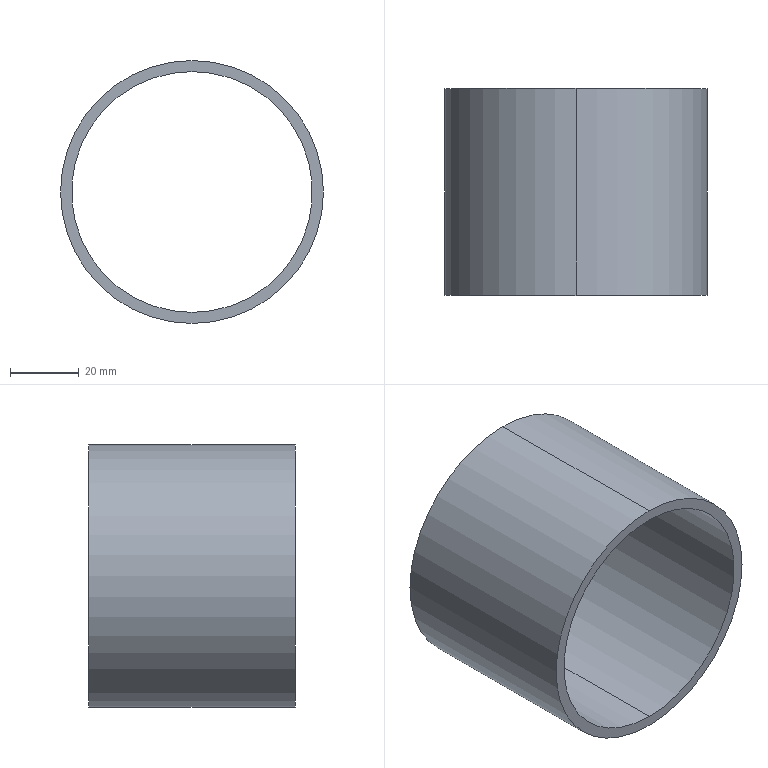Part | SolidWorks | features Extrusion 1 | 1 solid | 6 faces | box 76.3 x 60 x 76.3 mm | volume 44093 mm3 | cylinder 4 | plane 2 | commonest cylinder face diameters 69.9 x2 76.3 x2
STEP:
#1=CARTESIAN_POINT('',(0.,60.,-34.95));
#2=VERTEX_POINT('',#1);
#3=CARTESIAN_POINT('',(0.,60.,34.95));
#4=VERTEX_POINT('',#3);
#5=CARTESIAN_POINT('',(0.,60.,0.));
#6=DIRECTION('',(0.,1.,0.));
#7=DIRECTION('',(0.,0.,1.));
#8=AXIS2_PLACEMENT_3D('',#5,#6,#7);
#9=CIRCLE('',#8,34.95);
#10=EDGE_CURVE('',#2,#4,#9,.T.);
#11=ORIENTED_EDGE('',*,*,#10,.T.);
#12=CARTESIAN_POINT('',(0.,0.,34.95));
#13=VERTEX_POINT('',#12);
#14=CARTESIAN_POINT('',(0.,60.,34.95));
#15=DIRECTION('',(0.,-1.,0.));
#16=VECTOR('',#15,1000.);
#17=LINE('',#14,#16);
#18=EDGE_CURVE('',#4,#13,#17,.T.);
#19=ORIENTED_EDGE('',*,*,#18,.T.);
#20=CARTESIAN_POINT('',(0.,0.,-34.95));
#21=VERTEX_POINT('',#20);
#22=CARTESIAN_POINT('',(0.,0.,0.));
#23=DIRECTION('',(0.,1.,0.));
#24=DIRECTION('',(0.,0.,1.));
#25=AXIS2_PLACEMENT_3D('',#22,#23,#24);
#26=CIRCLE('',#25,34.95);
#27=EDGE_CURVE('',#21,#13,#26,.T.);
#28=ORIENTED_EDGE('',*,*,#27,.F.);
#29=CARTESIAN_POINT('',(0.,60.,-34.95));
#30=DIRECTION('',(0.,-1.,0.));
#31=VECTOR('',#30,1000.);
#32=LINE('',#29,#31);
#33=EDGE_CURVE('',#2,#21,#32,.T.);
#34=ORIENTED_EDGE('',*,*,#33,.F.);
#35=EDGE_LOOP('',(#11,#19,#28,#34));
#36=FACE_OUTER_BOUND('',#35,.T.);
#37=CARTESIAN_POINT('',(0.,60.,0.));
#38=DIRECTION('',(0.,-1.,0.));
#39=DIRECTION('',(0.,0.,-1.));
#40=AXIS2_PLACEMENT_3D('',#37,#38,#39);
#41=CYLINDRICAL_SURFACE('',#40,34.95);
#42=ADVANCED_FACE('',(#36),#41,.F.);
#43=CARTESIAN_POINT('',(0.,60.,38.15));
#44=VERTEX_POINT('',#43);
#45=CARTESIAN_POINT('',(0.,60.,-38.15));
#46=VERTEX_POINT('',#45);
#47=CARTESIAN_POINT('',(0.,60.,0.));
#48=DIRECTION('',(0.,1.,0.));
#49=DIRECTION('',(0.,0.,1.));
#50=AXIS2_PLACEMENT_3D('',#47,#48,#49);
#51=CIRCLE('',#50,38.15);
#52=EDGE_CURVE('',#44,#46,#51,.T.);
#53=ORIENTED_EDGE('',*,*,#52,.F.);
#54=CARTESIAN_POINT('',(0.,0.,38.15));
#55=VERTEX_POINT('',#54);
#56=CARTESIAN_POINT('',(0.,60.,38.15));
#57=DIRECTION('',(0.,-1.,0.));
#58=VECTOR('',#57,1000.);
#59=LINE('',#56,#58);
#60=EDGE_CURVE('',#44,#55,#59,.T.);
#61=ORIENTED_EDGE('',*,*,#60,.T.);
#62=CARTESIAN_POINT('',(0.,0.,-38.15));
#63=VERTEX_POINT('',#62);
#64=CARTESIAN_POINT('',(0.,0.,0.));
#65=DIRECTION('',(0.,1.,0.));
#66=DIRECTION('',(0.,0.,1.));
#67=AXIS2_PLACEMENT_3D('',#64,#65,#66);
#68=CIRCLE('',#67,38.15);
#69=EDGE_CURVE('',#55,#63,#68,.T.);
#70=ORIENTED_EDGE('',*,*,#69,.T.);
#71=CARTESIAN_POINT('',(0.,60.,-38.15));
#72=DIRECTION('',(0.,-1.,0.));
#73=VECTOR('',#72,1000.);
#74=LINE('',#71,#73);
#75=EDGE_CURVE('',#46,#63,#74,.T.);
#76=ORIENTED_EDGE('',*,*,#75,.F.);
#77=EDGE_LOOP('',(#53,#61,#70,#76));
#78=FACE_OUTER_BOUND('',#77,.T.);
#79=CARTESIAN_POINT('',(0.,60.,0.));
#80=DIRECTION('',(0.,-1.,0.));
#81=DIRECTION('',(0.,0.,-1.));
#82=AXIS2_PLACEMENT_3D('',#79,#80,#81);
#83=CYLINDRICAL_SURFACE('',#82,38.15);
#84=ADVANCED_FACE('',(#78),#83,.T.);
#85=CARTESIAN_POINT('',(0.,60.,0.));
#86=DIRECTION('',(0.,1.,0.));
#87=DIRECTION('',(0.,0.,1.));
#88=AXIS2_PLACEMENT_3D('',#85,#86,#87);
#89=CIRCLE('',#88,38.15);
#90=EDGE_CURVE('',#46,#44,#89,.T.);
#91=ORIENTED_EDGE('',*,*,#90,.T.);
#92=ORIENTED_EDGE('',*,*,#52,.T.);
#93=EDGE_LOOP('',(#91,#92));
#94=FACE_OUTER_BOUND('',#93,.T.);
#95=ORIENTED_EDGE('',*,*,#10,.F.);
#96=CARTESIAN_POINT('',(0.,60.,0.));
#97=DIRECTION('',(0.,1.,0.));
#98=DIRECTION('',(0.,0.,1.));
#99=AXIS2_PLACEMENT_3D('',#96,#97,#98);
#100=CIRCLE('',#99,34.95);
#101=EDGE_CURVE('',#4,#2,#100,.T.);
#102=ORIENTED_EDGE('',*,*,#101,.F.);
#103=EDGE_LOOP('',(#95,#102));
#104=FACE_BOUND('',#103,.T.);
#105=CARTESIAN_POINT('',(0.,60.,0.));
#106=DIRECTION('',(0.,1.,0.));
#107=DIRECTION('',(0.,0.,1.));
#108=AXIS2_PLACEMENT_3D('',#105,#106,#107);
#109=PLANE('',#108);
#110=ADVANCED_FACE('',(#94,#104),#109,.T.);
#111=CARTESIAN_POINT('',(0.,0.,0.));
#112=DIRECTION('',(0.,1.,0.));
#113=DIRECTION('',(0.,0.,1.));
#114=AXIS2_PLACEMENT_3D('',#111,#112,#113);
#115=CIRCLE('',#114,38.15);
#116=EDGE_CURVE('',#63,#55,#115,.T.);
#117=ORIENTED_EDGE('',*,*,#116,.F.);
#118=ORIENTED_EDGE('',*,*,#69,.F.);
#119=EDGE_LOOP('',(#117,#118));
#120=FACE_OUTER_BOUND('',#119,.T.);
#121=ORIENTED_EDGE('',*,*,#27,.T.);
#122=CARTESIAN_POINT('',(0.,0.,0.));
#123=DIRECTION('',(0.,1.,0.));
#124=DIRECTION('',(0.,0.,1.));
#125=AXIS2_PLACEMENT_3D('',#122,#123,#124);
#126=CIRCLE('',#125,34.95);
#127=EDGE_CURVE('',#13,#21,#126,.T.);
#128=ORIENTED_EDGE('',*,*,#127,.T.);
#129=EDGE_LOOP('',(#121,#128));
#130=FACE_BOUND('',#129,.T.);
#131=CARTESIAN_POINT('',(0.,0.,0.));
#132=DIRECTION('',(0.,1.,0.));
#133=DIRECTION('',(0.,0.,1.));
#134=AXIS2_PLACEMENT_3D('',#131,#132,#133);
#135=PLANE('',#134);
#136=ADVANCED_FACE('',(#120,#130),#135,.F.);
#137=ORIENTED_EDGE('',*,*,#60,.F.);
#138=ORIENTED_EDGE('',*,*,#90,.F.);
#139=ORIENTED_EDGE('',*,*,#75,.T.);
#140=ORIENTED_EDGE('',*,*,#116,.T.);
#141=EDGE_LOOP('',(#137,#138,#139,#140));
#142=FACE_OUTER_BOUND('',#141,.T.);
#143=CARTESIAN_POINT('',(0.,60.,0.));
#144=DIRECTION('',(0.,-1.,0.));
#145=DIRECTION('',(0.,0.,-1.));
#146=AXIS2_PLACEMENT_3D('',#143,#144,#145);
#147=CYLINDRICAL_SURFACE('',#146,38.15);
#148=ADVANCED_FACE('',(#142),#147,.T.);
#149=ORIENTED_EDGE('',*,*,#18,.F.);
#150=ORIENTED_EDGE('',*,*,#101,.T.);
#151=ORIENTED_EDGE('',*,*,#33,.T.);
#152=ORIENTED_EDGE('',*,*,#127,.F.);
#153=EDGE_LOOP('',(#149,#150,#151,#152));
#154=FACE_OUTER_BOUND('',#153,.T.);
#155=CARTESIAN_POINT('',(0.,60.,0.));
#156=DIRECTION('',(0.,-1.,0.));
#157=DIRECTION('',(0.,0.,-1.));
#158=AXIS2_PLACEMENT_3D('',#155,#156,#157);
#159=CYLINDRICAL_SURFACE('',#158,34.95);
#160=ADVANCED_FACE('',(#154),#159,.F.);
#161=CLOSED_SHELL('',(#42,#84,#110,#136,#148,#160));
#162=MANIFOLD_SOLID_BREP('',#161);
#163=CARTESIAN_POINT('',(0.,0.,0.));
#164=DIRECTION('',(0.,0.,1.));
#165=DIRECTION('',(1.,0.,0.));
#166=AXIS2_PLACEMENT_3D('',#163,#164,#165);
#167=(LENGTH_UNIT()NAMED_UNIT(*)SI_UNIT(.MILLI.,.METRE.));
#168=UNCERTAINTY_MEASURE_WITH_UNIT(LENGTH_MEASURE(0.00001),#167,'','');
#169=(NAMED_UNIT(*)PLANE_ANGLE_UNIT()SI_UNIT($,.RADIAN.));
#170=(NAMED_UNIT(*)SI_UNIT($,.STERADIAN.)SOLID_ANGLE_UNIT());
#171=(GEOMETRIC_REPRESENTATION_CONTEXT(3)GLOBAL_UNCERTAINTY_ASSIGNED_CONTEXT((#168))GLOBAL_UNIT_ASSIGNED_CONTEXT((#167,#169,#170))REPRESENTATION_CONTEXT('',''));
#172=ADVANCED_BREP_SHAPE_REPRESENTATION('',(#162,#166),#171);